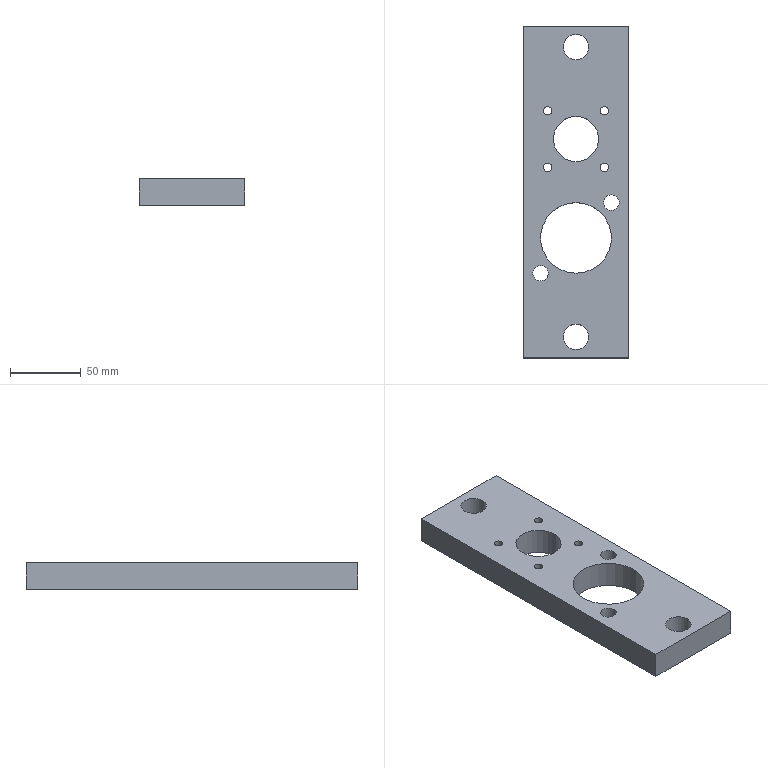Part | NX | features solid 2 | 1 solid | 16 faces | box 75 x 235 x 19 mm | volume 266858 mm3 | cylinder 10 | plane 6 | commonest cylinder face diameters 6 x4 11 x2 18 x2 32 x1 50 x1
STEP:
#1=CARTESIAN_POINT('',(-615.,-60.,-111.));
#2=VERTEX_POINT('',#1);
#3=CARTESIAN_POINT('',(-615.,-60.,-130.));
#4=VERTEX_POINT('',#3);
#5=CARTESIAN_POINT('',(-615.,-60.,-111.));
#6=DIRECTION('',(0.,0.,-1.));
#7=VECTOR('',#6,1000.);
#8=LINE('',#5,#7);
#9=EDGE_CURVE('',#2,#4,#8,.T.);
#10=ORIENTED_EDGE('',*,*,#9,.F.);
#11=CARTESIAN_POINT('',(-615.,-295.,-111.));
#12=VERTEX_POINT('',#11);
#13=CARTESIAN_POINT('',(-615.,-295.,-111.));
#14=DIRECTION('',(0.,1.,0.));
#15=VECTOR('',#14,1000.);
#16=LINE('',#13,#15);
#17=EDGE_CURVE('',#12,#2,#16,.T.);
#18=ORIENTED_EDGE('',*,*,#17,.F.);
#19=CARTESIAN_POINT('',(-615.,-295.,-130.));
#20=VERTEX_POINT('',#19);
#21=CARTESIAN_POINT('',(-615.,-295.,-111.));
#22=DIRECTION('',(0.,0.,-1.));
#23=VECTOR('',#22,1000.);
#24=LINE('',#21,#23);
#25=EDGE_CURVE('',#12,#20,#24,.T.);
#26=ORIENTED_EDGE('',*,*,#25,.T.);
#27=CARTESIAN_POINT('',(-615.,-295.,-130.));
#28=DIRECTION('',(0.,1.,0.));
#29=VECTOR('',#28,1000.);
#30=LINE('',#27,#29);
#31=EDGE_CURVE('',#20,#4,#30,.T.);
#32=ORIENTED_EDGE('',*,*,#31,.T.);
#33=EDGE_LOOP('',(#10,#18,#26,#32));
#34=FACE_BOUND('',#33,.T.);
#35=CARTESIAN_POINT('',(-615.,-295.,-111.));
#36=DIRECTION('',(-1.,0.,0.));
#37=DIRECTION('',(0.,0.,1.));
#38=AXIS2_PLACEMENT_3D('',#35,#36,#37);
#39=PLANE('',#38);
#40=ADVANCED_FACE('',(#34),#39,.F.);
#41=CARTESIAN_POINT('',(-690.,-60.,-130.));
#42=VERTEX_POINT('',#41);
#43=CARTESIAN_POINT('',(-690.,-60.,-111.));
#44=VERTEX_POINT('',#43);
#45=CARTESIAN_POINT('',(-690.,-60.,-111.));
#46=DIRECTION('',(0.,0.,1.));
#47=VECTOR('',#46,1000.);
#48=LINE('',#45,#47);
#49=EDGE_CURVE('',#42,#44,#48,.T.);
#50=ORIENTED_EDGE('',*,*,#49,.F.);
#51=CARTESIAN_POINT('',(-690.,-295.,-130.));
#52=VERTEX_POINT('',#51);
#53=CARTESIAN_POINT('',(-690.,15.,-130.));
#54=DIRECTION('',(0.,-1.,0.));
#55=VECTOR('',#54,1000.);
#56=LINE('',#53,#55);
#57=EDGE_CURVE('',#42,#52,#56,.T.);
#58=ORIENTED_EDGE('',*,*,#57,.T.);
#59=CARTESIAN_POINT('',(-690.,-295.,-111.));
#60=VERTEX_POINT('',#59);
#61=CARTESIAN_POINT('',(-690.,-295.,-111.));
#62=DIRECTION('',(0.,0.,-1.));
#63=VECTOR('',#62,1000.);
#64=LINE('',#61,#63);
#65=EDGE_CURVE('',#60,#52,#64,.T.);
#66=ORIENTED_EDGE('',*,*,#65,.F.);
#67=CARTESIAN_POINT('',(-690.,15.,-111.));
#68=DIRECTION('',(0.,-1.,0.));
#69=VECTOR('',#68,1000.);
#70=LINE('',#67,#69);
#71=EDGE_CURVE('',#44,#60,#70,.T.);
#72=ORIENTED_EDGE('',*,*,#71,.F.);
#73=EDGE_LOOP('',(#50,#58,#66,#72));
#74=FACE_BOUND('',#73,.T.);
#75=CARTESIAN_POINT('',(-690.,15.,-111.));
#76=DIRECTION('',(1.,0.,0.));
#77=DIRECTION('',(0.,0.,-1.));
#78=AXIS2_PLACEMENT_3D('',#75,#76,#77);
#79=PLANE('',#78);
#80=ADVANCED_FACE('',(#74),#79,.F.);
#81=CARTESIAN_POINT('',(-652.5,-66.,-111.));
#82=VERTEX_POINT('',#81);
#83=CARTESIAN_POINT('',(-652.5,-75.,-111.));
#84=DIRECTION('',(0.,0.,1.));
#85=DIRECTION('',(0.,1.,0.));
#86=AXIS2_PLACEMENT_3D('',#83,#84,#85);
#87=CIRCLE('',#86,9.);
#88=EDGE_CURVE('',#82,#82,#87,.T.);
#89=ORIENTED_EDGE('',*,*,#88,.F.);
#90=EDGE_LOOP('',(#89));
#91=FACE_BOUND('',#90,.T.);
#92=CARTESIAN_POINT('',(-652.5,-235.,-111.));
#93=VERTEX_POINT('',#92);
#94=CARTESIAN_POINT('',(-652.5,-210.,-111.));
#95=DIRECTION('',(0.,0.,-1.));
#96=DIRECTION('',(0.,-1.,0.));
#97=AXIS2_PLACEMENT_3D('',#94,#95,#96);
#98=CIRCLE('',#97,25.);
#99=EDGE_CURVE('',#93,#93,#98,.T.);
#100=ORIENTED_EDGE('',*,*,#99,.T.);
#101=EDGE_LOOP('',(#100));
#102=FACE_BOUND('',#101,.T.);
#103=CARTESIAN_POINT('',(-672.5,-117.,-111.));
#104=VERTEX_POINT('',#103);
#105=CARTESIAN_POINT('',(-672.5,-120.,-111.));
#106=DIRECTION('',(0.,0.,1.));
#107=DIRECTION('',(0.,1.,0.));
#108=AXIS2_PLACEMENT_3D('',#105,#106,#107);
#109=CIRCLE('',#108,3.);
#110=EDGE_CURVE('',#104,#104,#109,.T.);
#111=ORIENTED_EDGE('',*,*,#110,.F.);
#112=EDGE_LOOP('',(#111));
#113=FACE_BOUND('',#112,.T.);
#114=CARTESIAN_POINT('',(-632.5,-163.,-111.));
#115=VERTEX_POINT('',#114);
#116=CARTESIAN_POINT('',(-632.5,-160.,-111.));
#117=DIRECTION('',(0.,0.,1.));
#118=DIRECTION('',(0.,-1.,0.));
#119=AXIS2_PLACEMENT_3D('',#116,#117,#118);
#120=CIRCLE('',#119,3.);
#121=EDGE_CURVE('',#115,#115,#120,.T.);
#122=ORIENTED_EDGE('',*,*,#121,.F.);
#123=EDGE_LOOP('',(#122));
#124=FACE_BOUND('',#123,.T.);
#125=CARTESIAN_POINT('',(-632.5,-117.,-111.));
#126=VERTEX_POINT('',#125);
#127=CARTESIAN_POINT('',(-632.5,-120.,-111.));
#128=DIRECTION('',(0.,0.,-1.));
#129=DIRECTION('',(0.,1.,0.));
#130=AXIS2_PLACEMENT_3D('',#127,#128,#129);
#131=CIRCLE('',#130,3.);
#132=EDGE_CURVE('',#126,#126,#131,.T.);
#133=ORIENTED_EDGE('',*,*,#132,.T.);
#134=EDGE_LOOP('',(#133));
#135=FACE_BOUND('',#134,.T.);
#136=CARTESIAN_POINT('',(-672.5,-163.,-111.));
#137=VERTEX_POINT('',#136);
#138=CARTESIAN_POINT('',(-672.5,-160.,-111.));
#139=DIRECTION('',(0.,0.,-1.));
#140=DIRECTION('',(0.,-1.,0.));
#141=AXIS2_PLACEMENT_3D('',#138,#139,#140);
#142=CIRCLE('',#141,3.);
#143=EDGE_CURVE('',#137,#137,#142,.T.);
#144=ORIENTED_EDGE('',*,*,#143,.T.);
#145=EDGE_LOOP('',(#144));
#146=FACE_BOUND('',#145,.T.);
#147=CARTESIAN_POINT('',(-677.5,-240.5,-111.));
#148=VERTEX_POINT('',#147);
#149=CARTESIAN_POINT('',(-677.5,-235.,-111.));
#150=DIRECTION('',(0.,0.,-1.));
#151=DIRECTION('',(0.,-1.,0.));
#152=AXIS2_PLACEMENT_3D('',#149,#150,#151);
#153=CIRCLE('',#152,5.5);
#154=EDGE_CURVE('',#148,#148,#153,.T.);
#155=ORIENTED_EDGE('',*,*,#154,.T.);
#156=EDGE_LOOP('',(#155));
#157=FACE_BOUND('',#156,.T.);
#158=CARTESIAN_POINT('',(-652.5,-289.,-111.));
#159=VERTEX_POINT('',#158);
#160=CARTESIAN_POINT('',(-652.5,-280.,-111.));
#161=DIRECTION('',(0.,0.,-1.));
#162=DIRECTION('',(0.,-1.,0.));
#163=AXIS2_PLACEMENT_3D('',#160,#161,#162);
#164=CIRCLE('',#163,9.);
#165=EDGE_CURVE('',#159,#159,#164,.T.);
#166=ORIENTED_EDGE('',*,*,#165,.T.);
#167=EDGE_LOOP('',(#166));
#168=FACE_BOUND('',#167,.T.);
#169=CARTESIAN_POINT('',(-652.5,-124.,-111.));
#170=VERTEX_POINT('',#169);
#171=CARTESIAN_POINT('',(-652.5,-140.,-111.));
#172=DIRECTION('',(0.,0.,1.));
#173=DIRECTION('',(0.,1.,0.));
#174=AXIS2_PLACEMENT_3D('',#171,#172,#173);
#175=CIRCLE('',#174,16.);
#176=EDGE_CURVE('',#170,#170,#175,.T.);
#177=ORIENTED_EDGE('',*,*,#176,.F.);
#178=EDGE_LOOP('',(#177));
#179=FACE_BOUND('',#178,.T.);
#180=CARTESIAN_POINT('',(-627.5,-190.5,-111.));
#181=VERTEX_POINT('',#180);
#182=CARTESIAN_POINT('',(-627.5,-185.,-111.));
#183=DIRECTION('',(0.,0.,-1.));
#184=DIRECTION('',(0.,-1.,0.));
#185=AXIS2_PLACEMENT_3D('',#182,#183,#184);
#186=CIRCLE('',#185,5.5);
#187=EDGE_CURVE('',#181,#181,#186,.T.);
#188=ORIENTED_EDGE('',*,*,#187,.T.);
#189=EDGE_LOOP('',(#188));
#190=FACE_BOUND('',#189,.T.);
#191=ORIENTED_EDGE('',*,*,#17,.T.);
#192=CARTESIAN_POINT('',(-615.,-60.,-111.));
#193=DIRECTION('',(-1.,0.,0.));
#194=VECTOR('',#193,1000.);
#195=LINE('',#192,#194);
#196=EDGE_CURVE('',#2,#44,#195,.T.);
#197=ORIENTED_EDGE('',*,*,#196,.T.);
#198=ORIENTED_EDGE('',*,*,#71,.T.);
#199=CARTESIAN_POINT('',(-690.,-295.,-111.));
#200=DIRECTION('',(1.,0.,0.));
#201=VECTOR('',#200,1000.);
#202=LINE('',#199,#201);
#203=EDGE_CURVE('',#60,#12,#202,.T.);
#204=ORIENTED_EDGE('',*,*,#203,.T.);
#205=EDGE_LOOP('',(#191,#197,#198,#204));
#206=FACE_BOUND('',#205,.T.);
#207=CARTESIAN_POINT('',(-615.,15.,-111.));
#208=DIRECTION('',(0.,0.,1.));
#209=DIRECTION('',(0.,1.,0.));
#210=AXIS2_PLACEMENT_3D('',#207,#208,#209);
#211=PLANE('',#210);
#212=ADVANCED_FACE('',(#91,#102,#113,#124,#135,#146,#157,#168,#179,#190,#206),#211,.T.);
#213=CARTESIAN_POINT('',(-652.5,-66.,-130.));
#214=VERTEX_POINT('',#213);
#215=CARTESIAN_POINT('',(-652.5,-75.,-130.));
#216=DIRECTION('',(0.,0.,1.));
#217=DIRECTION('',(0.,1.,0.));
#218=AXIS2_PLACEMENT_3D('',#215,#216,#217);
#219=CIRCLE('',#218,9.);
#220=EDGE_CURVE('',#214,#214,#219,.T.);
#221=ORIENTED_EDGE('',*,*,#220,.T.);
#222=EDGE_LOOP('',(#221));
#223=FACE_BOUND('',#222,.T.);
#224=CARTESIAN_POINT('',(-652.5,-235.,-130.));
#225=VERTEX_POINT('',#224);
#226=CARTESIAN_POINT('',(-652.5,-210.,-130.));
#227=DIRECTION('',(0.,0.,-1.));
#228=DIRECTION('',(0.,-1.,0.));
#229=AXIS2_PLACEMENT_3D('',#226,#227,#228);
#230=CIRCLE('',#229,25.);
#231=EDGE_CURVE('',#225,#225,#230,.T.);
#232=ORIENTED_EDGE('',*,*,#231,.F.);
#233=EDGE_LOOP('',(#232));
#234=FACE_BOUND('',#233,.T.);
#235=CARTESIAN_POINT('',(-672.5,-117.,-130.));
#236=VERTEX_POINT('',#235);
#237=CARTESIAN_POINT('',(-672.5,-120.,-130.));
#238=DIRECTION('',(0.,0.,1.));
#239=DIRECTION('',(0.,1.,0.));
#240=AXIS2_PLACEMENT_3D('',#237,#238,#239);
#241=CIRCLE('',#240,3.);
#242=EDGE_CURVE('',#236,#236,#241,.T.);
#243=ORIENTED_EDGE('',*,*,#242,.T.);
#244=EDGE_LOOP('',(#243));
#245=FACE_BOUND('',#244,.T.);
#246=CARTESIAN_POINT('',(-632.5,-163.,-130.));
#247=VERTEX_POINT('',#246);
#248=CARTESIAN_POINT('',(-632.5,-160.,-130.));
#249=DIRECTION('',(0.,0.,1.));
#250=DIRECTION('',(0.,-1.,0.));
#251=AXIS2_PLACEMENT_3D('',#248,#249,#250);
#252=CIRCLE('',#251,3.);
#253=EDGE_CURVE('',#247,#247,#252,.T.);
#254=ORIENTED_EDGE('',*,*,#253,.T.);
#255=EDGE_LOOP('',(#254));
#256=FACE_BOUND('',#255,.T.);
#257=CARTESIAN_POINT('',(-632.5,-117.,-130.));
#258=VERTEX_POINT('',#257);
#259=CARTESIAN_POINT('',(-632.5,-120.,-130.));
#260=DIRECTION('',(0.,0.,-1.));
#261=DIRECTION('',(0.,1.,0.));
#262=AXIS2_PLACEMENT_3D('',#259,#260,#261);
#263=CIRCLE('',#262,3.);
#264=EDGE_CURVE('',#258,#258,#263,.T.);
#265=ORIENTED_EDGE('',*,*,#264,.F.);
#266=EDGE_LOOP('',(#265));
#267=FACE_BOUND('',#266,.T.);
#268=CARTESIAN_POINT('',(-672.5,-163.,-130.));
#269=VERTEX_POINT('',#268);
#270=CARTESIAN_POINT('',(-672.5,-160.,-130.));
#271=DIRECTION('',(0.,0.,-1.));
#272=DIRECTION('',(0.,-1.,0.));
#273=AXIS2_PLACEMENT_3D('',#270,#271,#272);
#274=CIRCLE('',#273,3.);
#275=EDGE_CURVE('',#269,#269,#274,.T.);
#276=ORIENTED_EDGE('',*,*,#275,.F.);
#277=EDGE_LOOP('',(#276));
#278=FACE_BOUND('',#277,.T.);
#279=CARTESIAN_POINT('',(-677.5,-240.5,-130.));
#280=VERTEX_POINT('',#279);
#281=CARTESIAN_POINT('',(-677.5,-235.,-130.));
#282=DIRECTION('',(0.,0.,-1.));
#283=DIRECTION('',(0.,-1.,0.));
#284=AXIS2_PLACEMENT_3D('',#281,#282,#283);
#285=CIRCLE('',#284,5.5);
#286=EDGE_CURVE('',#280,#280,#285,.T.);
#287=ORIENTED_EDGE('',*,*,#286,.F.);
#288=EDGE_LOOP('',(#287));
#289=FACE_BOUND('',#288,.T.);
#290=CARTESIAN_POINT('',(-652.5,-289.,-130.));
#291=VERTEX_POINT('',#290);
#292=CARTESIAN_POINT('',(-652.5,-280.,-130.));
#293=DIRECTION('',(0.,0.,-1.));
#294=DIRECTION('',(0.,-1.,0.));
#295=AXIS2_PLACEMENT_3D('',#292,#293,#294);
#296=CIRCLE('',#295,9.);
#297=EDGE_CURVE('',#291,#291,#296,.T.);
#298=ORIENTED_EDGE('',*,*,#297,.F.);
#299=EDGE_LOOP('',(#298));
#300=FACE_BOUND('',#299,.T.);
#301=CARTESIAN_POINT('',(-652.5,-124.,-130.));
#302=VERTEX_POINT('',#301);
#303=CARTESIAN_POINT('',(-652.5,-140.,-130.));
#304=DIRECTION('',(0.,0.,1.));
#305=DIRECTION('',(0.,1.,0.));
#306=AXIS2_PLACEMENT_3D('',#303,#304,#305);
#307=CIRCLE('',#306,16.);
#308=EDGE_CURVE('',#302,#302,#307,.T.);
#309=ORIENTED_EDGE('',*,*,#308,.T.);
#310=EDGE_LOOP('',(#309));
#311=FACE_BOUND('',#310,.T.);
#312=CARTESIAN_POINT('',(-627.5,-190.5,-130.));
#313=VERTEX_POINT('',#312);
#314=CARTESIAN_POINT('',(-627.5,-185.,-130.));
#315=DIRECTION('',(0.,0.,-1.));
#316=DIRECTION('',(0.,-1.,0.));
#317=AXIS2_PLACEMENT_3D('',#314,#315,#316);
#318=CIRCLE('',#317,5.5);
#319=EDGE_CURVE('',#313,#313,#318,.T.);
#320=ORIENTED_EDGE('',*,*,#319,.F.);
#321=EDGE_LOOP('',(#320));
#322=FACE_BOUND('',#321,.T.);
#323=CARTESIAN_POINT('',(-615.,-60.,-130.));
#324=DIRECTION('',(-1.,0.,0.));
#325=VECTOR('',#324,1000.);
#326=LINE('',#323,#325);
#327=EDGE_CURVE('',#4,#42,#326,.T.);
#328=ORIENTED_EDGE('',*,*,#327,.F.);
#329=ORIENTED_EDGE('',*,*,#31,.F.);
#330=CARTESIAN_POINT('',(-690.,-295.,-130.));
#331=DIRECTION('',(1.,0.,0.));
#332=VECTOR('',#331,1000.);
#333=LINE('',#330,#332);
#334=EDGE_CURVE('',#52,#20,#333,.T.);
#335=ORIENTED_EDGE('',*,*,#334,.F.);
#336=ORIENTED_EDGE('',*,*,#57,.F.);
#337=EDGE_LOOP('',(#328,#329,#335,#336));
#338=FACE_BOUND('',#337,.T.);
#339=CARTESIAN_POINT('',(-615.,15.,-130.));
#340=DIRECTION('',(0.,0.,1.));
#341=DIRECTION('',(0.,1.,0.));
#342=AXIS2_PLACEMENT_3D('',#339,#340,#341);
#343=PLANE('',#342);
#344=ADVANCED_FACE('',(#223,#234,#245,#256,#267,#278,#289,#300,#311,#322,#338),#343,.F.);
#345=ORIENTED_EDGE('',*,*,#110,.T.);
#346=EDGE_LOOP('',(#345));
#347=FACE_BOUND('',#346,.T.);
#348=ORIENTED_EDGE('',*,*,#242,.F.);
#349=EDGE_LOOP('',(#348));
#350=FACE_BOUND('',#349,.T.);
#351=CARTESIAN_POINT('',(-672.5,-120.,-111.));
#352=DIRECTION('',(0.,0.,-1.));
#353=DIRECTION('',(0.,-1.,0.));
#354=AXIS2_PLACEMENT_3D('',#351,#352,#353);
#355=CYLINDRICAL_SURFACE('',#354,3.);
#356=ADVANCED_FACE('',(#347,#350),#355,.F.);
#357=ORIENTED_EDGE('',*,*,#121,.T.);
#358=EDGE_LOOP('',(#357));
#359=FACE_BOUND('',#358,.T.);
#360=ORIENTED_EDGE('',*,*,#253,.F.);
#361=EDGE_LOOP('',(#360));
#362=FACE_BOUND('',#361,.T.);
#363=CARTESIAN_POINT('',(-632.5,-160.,-111.));
#364=DIRECTION('',(0.,0.,-1.));
#365=DIRECTION('',(0.,-1.,0.));
#366=AXIS2_PLACEMENT_3D('',#363,#364,#365);
#367=CYLINDRICAL_SURFACE('',#366,3.);
#368=ADVANCED_FACE('',(#359,#362),#367,.F.);
#369=ORIENTED_EDGE('',*,*,#132,.F.);
#370=EDGE_LOOP('',(#369));
#371=FACE_BOUND('',#370,.T.);
#372=ORIENTED_EDGE('',*,*,#264,.T.);
#373=EDGE_LOOP('',(#372));
#374=FACE_BOUND('',#373,.T.);
#375=CARTESIAN_POINT('',(-632.5,-120.,-111.));
#376=DIRECTION('',(0.,0.,-1.));
#377=DIRECTION('',(0.,-1.,0.));
#378=AXIS2_PLACEMENT_3D('',#375,#376,#377);
#379=CYLINDRICAL_SURFACE('',#378,3.);
#380=ADVANCED_FACE('',(#371,#374),#379,.F.);
#381=ORIENTED_EDGE('',*,*,#143,.F.);
#382=EDGE_LOOP('',(#381));
#383=FACE_BOUND('',#382,.T.);
#384=ORIENTED_EDGE('',*,*,#275,.T.);
#385=EDGE_LOOP('',(#384));
#386=FACE_BOUND('',#385,.T.);
#387=CARTESIAN_POINT('',(-672.5,-160.,-111.));
#388=DIRECTION('',(0.,0.,-1.));
#389=DIRECTION('',(0.,-1.,0.));
#390=AXIS2_PLACEMENT_3D('',#387,#388,#389);
#391=CYLINDRICAL_SURFACE('',#390,3.);
#392=ADVANCED_FACE('',(#383,#386),#391,.F.);
#393=ORIENTED_EDGE('',*,*,#334,.T.);
#394=ORIENTED_EDGE('',*,*,#25,.F.);
#395=ORIENTED_EDGE('',*,*,#203,.F.);
#396=ORIENTED_EDGE('',*,*,#65,.T.);
#397=EDGE_LOOP('',(#393,#394,#395,#396));
#398=FACE_BOUND('',#397,.T.);
#399=CARTESIAN_POINT('',(-690.,-295.,-111.));
#400=DIRECTION('',(0.,1.,0.));
#401=DIRECTION('',(0.,0.,-1.));
#402=AXIS2_PLACEMENT_3D('',#399,#400,#401);
#403=PLANE('',#402);
#404=ADVANCED_FACE('',(#398),#403,.F.);
#405=ORIENTED_EDGE('',*,*,#154,.F.);
#406=EDGE_LOOP('',(#405));
#407=FACE_BOUND('',#406,.T.);
#408=ORIENTED_EDGE('',*,*,#286,.T.);
#409=EDGE_LOOP('',(#408));
#410=FACE_BOUND('',#409,.T.);
#411=CARTESIAN_POINT('',(-677.5,-235.,-111.));
#412=DIRECTION('',(0.,0.,-1.));
#413=DIRECTION('',(0.,-1.,0.));
#414=AXIS2_PLACEMENT_3D('',#411,#412,#413);
#415=CYLINDRICAL_SURFACE('',#414,5.5);
#416=ADVANCED_FACE('',(#407,#410),#415,.F.);
#417=ORIENTED_EDGE('',*,*,#165,.F.);
#418=EDGE_LOOP('',(#417));
#419=FACE_BOUND('',#418,.T.);
#420=ORIENTED_EDGE('',*,*,#297,.T.);
#421=EDGE_LOOP('',(#420));
#422=FACE_BOUND('',#421,.T.);
#423=CARTESIAN_POINT('',(-652.5,-280.,-111.));
#424=DIRECTION('',(0.,0.,-1.));
#425=DIRECTION('',(0.,-1.,0.));
#426=AXIS2_PLACEMENT_3D('',#423,#424,#425);
#427=CYLINDRICAL_SURFACE('',#426,9.);
#428=ADVANCED_FACE('',(#419,#422),#427,.F.);
#429=ORIENTED_EDGE('',*,*,#176,.T.);
#430=EDGE_LOOP('',(#429));
#431=FACE_BOUND('',#430,.T.);
#432=ORIENTED_EDGE('',*,*,#308,.F.);
#433=EDGE_LOOP('',(#432));
#434=FACE_BOUND('',#433,.T.);
#435=CARTESIAN_POINT('',(-652.5,-140.,-111.));
#436=DIRECTION('',(0.,0.,-1.));
#437=DIRECTION('',(0.,-1.,0.));
#438=AXIS2_PLACEMENT_3D('',#435,#436,#437);
#439=CYLINDRICAL_SURFACE('',#438,16.);
#440=ADVANCED_FACE('',(#431,#434),#439,.F.);
#441=ORIENTED_EDGE('',*,*,#187,.F.);
#442=EDGE_LOOP('',(#441));
#443=FACE_BOUND('',#442,.T.);
#444=ORIENTED_EDGE('',*,*,#319,.T.);
#445=EDGE_LOOP('',(#444));
#446=FACE_BOUND('',#445,.T.);
#447=CARTESIAN_POINT('',(-627.5,-185.,-111.));
#448=DIRECTION('',(0.,0.,-1.));
#449=DIRECTION('',(0.,-1.,0.));
#450=AXIS2_PLACEMENT_3D('',#447,#448,#449);
#451=CYLINDRICAL_SURFACE('',#450,5.5);
#452=ADVANCED_FACE('',(#443,#446),#451,.F.);
#453=ORIENTED_EDGE('',*,*,#99,.F.);
#454=EDGE_LOOP('',(#453));
#455=FACE_BOUND('',#454,.T.);
#456=ORIENTED_EDGE('',*,*,#231,.T.);
#457=EDGE_LOOP('',(#456));
#458=FACE_BOUND('',#457,.T.);
#459=CARTESIAN_POINT('',(-652.5,-210.,-111.));
#460=DIRECTION('',(0.,0.,-1.));
#461=DIRECTION('',(0.,-1.,0.));
#462=AXIS2_PLACEMENT_3D('',#459,#460,#461);
#463=CYLINDRICAL_SURFACE('',#462,25.);
#464=ADVANCED_FACE('',(#455,#458),#463,.F.);
#465=ORIENTED_EDGE('',*,*,#196,.F.);
#466=ORIENTED_EDGE('',*,*,#9,.T.);
#467=ORIENTED_EDGE('',*,*,#327,.T.);
#468=ORIENTED_EDGE('',*,*,#49,.T.);
#469=EDGE_LOOP('',(#465,#466,#467,#468));
#470=FACE_BOUND('',#469,.T.);
#471=CARTESIAN_POINT('',(-652.5,-60.,-147.5));
#472=DIRECTION('',(0.,1.,0.));
#473=DIRECTION('',(-1.,0.,0.));
#474=AXIS2_PLACEMENT_3D('',#471,#472,#473);
#475=PLANE('',#474);
#476=ADVANCED_FACE('',(#470),#475,.T.);
#477=ORIENTED_EDGE('',*,*,#88,.T.);
#478=EDGE_LOOP('',(#477));
#479=FACE_BOUND('',#478,.T.);
#480=ORIENTED_EDGE('',*,*,#220,.F.);
#481=EDGE_LOOP('',(#480));
#482=FACE_BOUND('',#481,.T.);
#483=CARTESIAN_POINT('',(-652.5,-75.,-111.));
#484=DIRECTION('',(0.,0.,-1.));
#485=DIRECTION('',(0.,1.,0.));
#486=AXIS2_PLACEMENT_3D('',#483,#484,#485);
#487=CYLINDRICAL_SURFACE('',#486,9.);
#488=ADVANCED_FACE('',(#479,#482),#487,.F.);
#489=CLOSED_SHELL('',(#40,#80,#212,#344,#356,#368,#380,#392,#404,#416,#428,#440,#452,#464,#476,#488));
#490=MANIFOLD_SOLID_BREP('',#489);
#491=(LENGTH_UNIT()NAMED_UNIT(*)SI_UNIT(.MILLI.,.METRE.));
#492=UNCERTAINTY_MEASURE_WITH_UNIT(LENGTH_MEASURE(0.00001),#491,'','');
#493=(NAMED_UNIT(*)PLANE_ANGLE_UNIT()SI_UNIT($,.RADIAN.));
#494=(NAMED_UNIT(*)SI_UNIT($,.STERADIAN.)SOLID_ANGLE_UNIT());
#495=(GEOMETRIC_REPRESENTATION_CONTEXT(3)GLOBAL_UNCERTAINTY_ASSIGNED_CONTEXT((#492))GLOBAL_UNIT_ASSIGNED_CONTEXT((#491,#493,#494))REPRESENTATION_CONTEXT('',''));
#496=ADVANCED_BREP_SHAPE_REPRESENTATION('',(#490),#495);